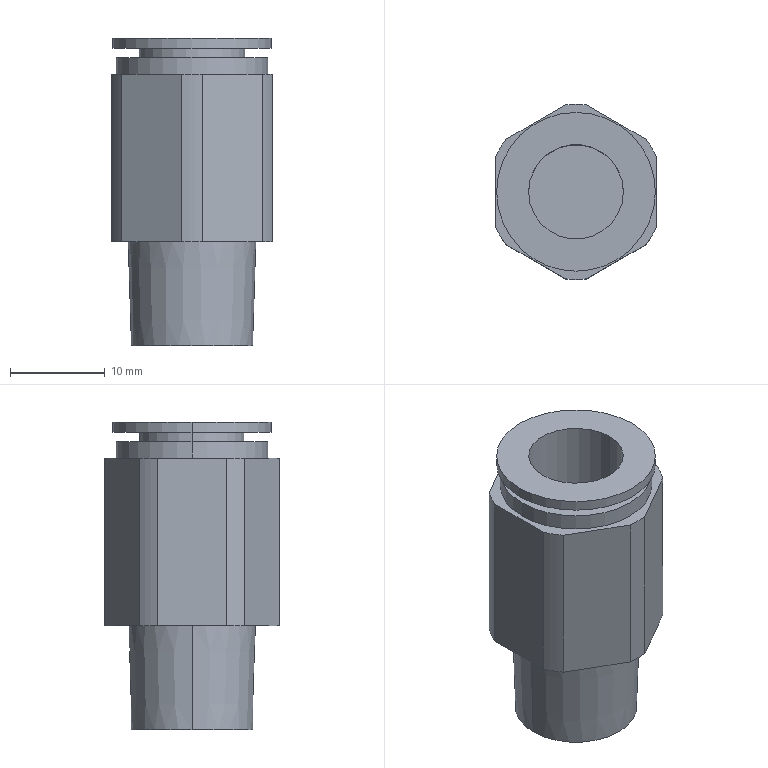Part | STEP file | GWS10-8 | 1 solid | 29 faces | box 17 x 18.5 x 32.5 mm | volume 4848 mm3 | cylinder 14 | plane 13 | cone 2 | commonest cylinder face diameters 18.5 x6 10 x2 11.1 x2 16 x2 16.75 x2